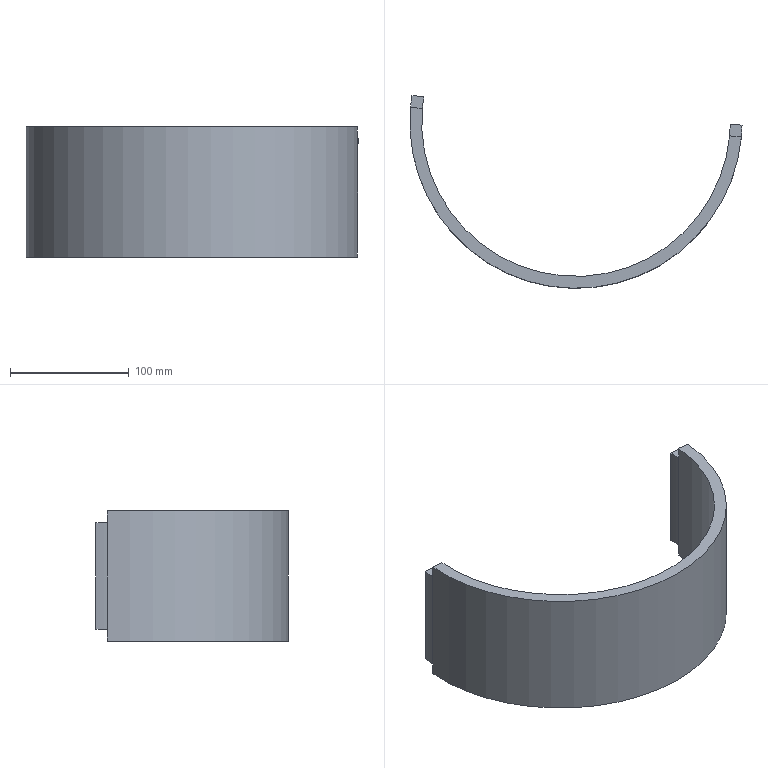Part | SolidWorks | features BaseBody 1 | 1 solid | 18 faces | box 279.978 x 162.405 x 110 mm | volume 484543 mm3 | plane 12 | cylinder 6 | commonest cylinder face diameters 260 x3 280 x3
STEP:
#1=CARTESIAN_POINT('',(399.859,1040.663,-284.893));
#2=VERTEX_POINT('',#1);
#3=CARTESIAN_POINT('',(389.899,1041.555,-284.893));
#4=VERTEX_POINT('',#3);
#5=CARTESIAN_POINT('',(946.393,991.761,-284.893));
#6=DIRECTION('',(-0.996,0.08912,0.));
#7=VECTOR('',#6,1000.);
#8=LINE('',#5,#7);
#9=EDGE_CURVE('',#2,#4,#8,.T.);
#10=ORIENTED_EDGE('',*,*,#9,.F.);
#11=CARTESIAN_POINT('',(399.859,1040.663,-294.893));
#12=VERTEX_POINT('',#11);
#13=CARTESIAN_POINT('',(399.859,1040.663,-184.893));
#14=DIRECTION('',(0.,0.,-1.));
#15=VECTOR('',#14,1000.);
#16=LINE('',#13,#15);
#17=EDGE_CURVE('',#2,#12,#16,.T.);
#18=ORIENTED_EDGE('',*,*,#17,.T.);
#19=CARTESIAN_POINT('',(389.899,1041.555,-294.893));
#20=VERTEX_POINT('',#19);
#21=CARTESIAN_POINT('',(260.416,1053.14,-294.893));
#22=DIRECTION('',(-0.996,0.08912,0.));
#23=VECTOR('',#22,1000.);
#24=LINE('',#21,#23);
#25=EDGE_CURVE('',#12,#20,#24,.T.);
#26=ORIENTED_EDGE('',*,*,#25,.T.);
#27=CARTESIAN_POINT('',(389.899,1041.555,-184.893));
#28=DIRECTION('',(0.,0.,-1.));
#29=VECTOR('',#28,1000.);
#30=LINE('',#27,#29);
#31=EDGE_CURVE('',#4,#20,#30,.T.);
#32=ORIENTED_EDGE('',*,*,#31,.F.);
#33=EDGE_LOOP('',(#10,#18,#26,#32));
#34=FACE_OUTER_BOUND('',#33,.T.);
#35=CARTESIAN_POINT('',(946.393,991.761,-284.893));
#36=DIRECTION('',(0.08912,0.996,0.));
#37=DIRECTION('',(0.,0.,-1.));
#38=AXIS2_PLACEMENT_3D('',#35,#36,#37);
#39=PLANE('',#38);
#40=ADVANCED_FACE('',(#34),#39,.T.);
#41=CARTESIAN_POINT('',(400.394,1050.655,-284.893));
#42=VERTEX_POINT('',#41);
#43=CARTESIAN_POINT('',(390.406,1051.549,-284.893));
#44=VERTEX_POINT('',#43);
#45=CARTESIAN_POINT('',(947.285,1001.721,-284.893));
#46=DIRECTION('',(-0.996,0.08912,0.));
#47=VECTOR('',#46,1000.);
#48=LINE('',#45,#47);
#49=EDGE_CURVE('',#42,#44,#48,.T.);
#50=ORIENTED_EDGE('',*,*,#49,.F.);
#51=CARTESIAN_POINT('',(260.416,1053.14,-284.893));
#52=DIRECTION('',(0.,0.,-1.));
#53=DIRECTION('',(0.08912,0.996,0.));
#54=AXIS2_PLACEMENT_3D('',#51,#52,#53);
#55=CIRCLE('',#54,140.);
#56=EDGE_CURVE('',#42,#2,#55,.T.);
#57=ORIENTED_EDGE('',*,*,#56,.T.);
#58=ORIENTED_EDGE('',*,*,#9,.T.);
#59=CARTESIAN_POINT('',(260.416,1053.14,-284.893));
#60=DIRECTION('',(0.,0.,-1.));
#61=DIRECTION('',(0.08912,0.996,0.));
#62=AXIS2_PLACEMENT_3D('',#59,#60,#61);
#63=CIRCLE('',#62,130.);
#64=EDGE_CURVE('',#44,#4,#63,.T.);
#65=ORIENTED_EDGE('',*,*,#64,.F.);
#66=EDGE_LOOP('',(#50,#57,#58,#65));
#67=FACE_OUTER_BOUND('',#66,.T.);
#68=CARTESIAN_POINT('',(946.393,991.761,-284.893));
#69=DIRECTION('',(0.,0.,-1.));
#70=DIRECTION('',(0.,-1.,0.));
#71=AXIS2_PLACEMENT_3D('',#68,#69,#70);
#72=PLANE('',#71);
#73=ADVANCED_FACE('',(#67),#72,.T.);
#74=CARTESIAN_POINT('',(400.394,1050.655,-194.893));
#75=VERTEX_POINT('',#74);
#76=CARTESIAN_POINT('',(390.406,1051.549,-194.893));
#77=VERTEX_POINT('',#76);
#78=CARTESIAN_POINT('',(947.285,1001.721,-194.893));
#79=DIRECTION('',(-0.996,0.08912,0.));
#80=VECTOR('',#79,1000.);
#81=LINE('',#78,#80);
#82=EDGE_CURVE('',#75,#77,#81,.T.);
#83=ORIENTED_EDGE('',*,*,#82,.F.);
#84=CARTESIAN_POINT('',(400.394,1050.655,-184.893));
#85=DIRECTION('',(0.,0.,-1.));
#86=VECTOR('',#85,1000.);
#87=LINE('',#84,#86);
#88=EDGE_CURVE('',#75,#42,#87,.T.);
#89=ORIENTED_EDGE('',*,*,#88,.T.);
#90=ORIENTED_EDGE('',*,*,#49,.T.);
#91=CARTESIAN_POINT('',(390.406,1051.549,-184.893));
#92=DIRECTION('',(0.,0.,-1.));
#93=VECTOR('',#92,1000.);
#94=LINE('',#91,#93);
#95=EDGE_CURVE('',#77,#44,#94,.T.);
#96=ORIENTED_EDGE('',*,*,#95,.F.);
#97=EDGE_LOOP('',(#83,#89,#90,#96));
#98=FACE_OUTER_BOUND('',#97,.T.);
#99=CARTESIAN_POINT('',(947.285,1001.721,-194.893));
#100=DIRECTION('',(0.08912,0.996,0.));
#101=DIRECTION('',(0.,0.,-1.));
#102=AXIS2_PLACEMENT_3D('',#99,#100,#101);
#103=PLANE('',#102);
#104=ADVANCED_FACE('',(#98),#103,.T.);
#105=CARTESIAN_POINT('',(399.859,1040.663,-194.893));
#106=VERTEX_POINT('',#105);
#107=CARTESIAN_POINT('',(389.899,1041.555,-194.893));
#108=VERTEX_POINT('',#107);
#109=CARTESIAN_POINT('',(946.393,991.761,-194.893));
#110=DIRECTION('',(-0.996,0.08912,0.));
#111=VECTOR('',#110,1000.);
#112=LINE('',#109,#111);
#113=EDGE_CURVE('',#106,#108,#112,.T.);
#114=ORIENTED_EDGE('',*,*,#113,.F.);
#115=CARTESIAN_POINT('',(260.416,1053.14,-194.893));
#116=DIRECTION('',(0.,0.,1.));
#117=DIRECTION('',(0.996,-0.08912,0.));
#118=AXIS2_PLACEMENT_3D('',#115,#116,#117);
#119=CIRCLE('',#118,140.);
#120=EDGE_CURVE('',#106,#75,#119,.T.);
#121=ORIENTED_EDGE('',*,*,#120,.T.);
#122=ORIENTED_EDGE('',*,*,#82,.T.);
#123=CARTESIAN_POINT('',(260.416,1053.14,-194.893));
#124=DIRECTION('',(0.,0.,1.));
#125=DIRECTION('',(0.996,-0.08912,0.));
#126=AXIS2_PLACEMENT_3D('',#123,#124,#125);
#127=CIRCLE('',#126,130.);
#128=EDGE_CURVE('',#108,#77,#127,.T.);
#129=ORIENTED_EDGE('',*,*,#128,.F.);
#130=EDGE_LOOP('',(#114,#121,#122,#129));
#131=FACE_OUTER_BOUND('',#130,.T.);
#132=CARTESIAN_POINT('',(947.285,1001.721,-194.893));
#133=DIRECTION('',(0.,0.,1.));
#134=DIRECTION('',(1.,0.,0.));
#135=AXIS2_PLACEMENT_3D('',#132,#133,#134);
#136=PLANE('',#135);
#137=ADVANCED_FACE('',(#131),#136,.T.);
#138=CARTESIAN_POINT('',(399.859,1040.663,-184.893));
#139=VERTEX_POINT('',#138);
#140=CARTESIAN_POINT('',(389.899,1041.555,-184.893));
#141=VERTEX_POINT('',#140);
#142=CARTESIAN_POINT('',(260.416,1053.14,-184.893));
#143=DIRECTION('',(-0.996,0.08912,0.));
#144=VECTOR('',#143,1000.);
#145=LINE('',#142,#144);
#146=EDGE_CURVE('',#139,#141,#145,.T.);
#147=ORIENTED_EDGE('',*,*,#146,.F.);
#148=CARTESIAN_POINT('',(399.859,1040.663,-184.893));
#149=DIRECTION('',(0.,0.,-1.));
#150=VECTOR('',#149,1000.);
#151=LINE('',#148,#150);
#152=EDGE_CURVE('',#139,#106,#151,.T.);
#153=ORIENTED_EDGE('',*,*,#152,.T.);
#154=ORIENTED_EDGE('',*,*,#113,.T.);
#155=CARTESIAN_POINT('',(389.899,1041.555,-184.893));
#156=DIRECTION('',(0.,0.,-1.));
#157=VECTOR('',#156,1000.);
#158=LINE('',#155,#157);
#159=EDGE_CURVE('',#141,#108,#158,.T.);
#160=ORIENTED_EDGE('',*,*,#159,.F.);
#161=EDGE_LOOP('',(#147,#153,#154,#160));
#162=FACE_OUTER_BOUND('',#161,.T.);
#163=CARTESIAN_POINT('',(946.393,991.761,-112.946));
#164=DIRECTION('',(0.08912,0.996,0.));
#165=DIRECTION('',(0.,0.,-1.));
#166=AXIS2_PLACEMENT_3D('',#163,#164,#165);
#167=PLANE('',#166);
#168=ADVANCED_FACE('',(#162),#167,.T.);
#169=CARTESIAN_POINT('',(130.933,1064.726,-194.893));
#170=VERTEX_POINT('',#169);
#171=CARTESIAN_POINT('',(120.973,1065.617,-194.893));
#172=VERTEX_POINT('',#171);
#173=CARTESIAN_POINT('',(946.393,991.761,-194.893));
#174=DIRECTION('',(-0.996,0.08912,0.));
#175=VECTOR('',#174,1000.);
#176=LINE('',#173,#175);
#177=EDGE_CURVE('',#170,#172,#176,.T.);
#178=ORIENTED_EDGE('',*,*,#177,.T.);
#179=CARTESIAN_POINT('',(120.973,1065.617,-184.893));
#180=VERTEX_POINT('',#179);
#181=CARTESIAN_POINT('',(120.973,1065.617,-184.893));
#182=DIRECTION('',(0.,0.,1.));
#183=VECTOR('',#182,1000.);
#184=LINE('',#181,#183);
#185=EDGE_CURVE('',#172,#180,#184,.T.);
#186=ORIENTED_EDGE('',*,*,#185,.T.);
#187=CARTESIAN_POINT('',(130.933,1064.726,-184.893));
#188=VERTEX_POINT('',#187);
#189=CARTESIAN_POINT('',(260.416,1053.14,-184.893));
#190=DIRECTION('',(-0.996,0.08912,0.));
#191=VECTOR('',#190,1000.);
#192=LINE('',#189,#191);
#193=EDGE_CURVE('',#188,#180,#192,.T.);
#194=ORIENTED_EDGE('',*,*,#193,.F.);
#195=CARTESIAN_POINT('',(130.933,1064.726,-184.893));
#196=DIRECTION('',(0.,0.,1.));
#197=VECTOR('',#196,1000.);
#198=LINE('',#195,#197);
#199=EDGE_CURVE('',#170,#188,#198,.T.);
#200=ORIENTED_EDGE('',*,*,#199,.F.);
#201=EDGE_LOOP('',(#178,#186,#194,#200));
#202=FACE_OUTER_BOUND('',#201,.T.);
#203=CARTESIAN_POINT('',(946.393,991.761,-112.946));
#204=DIRECTION('',(0.08912,0.996,0.));
#205=DIRECTION('',(0.,0.,-1.));
#206=AXIS2_PLACEMENT_3D('',#203,#204,#205);
#207=PLANE('',#206);
#208=ADVANCED_FACE('',(#202),#207,.T.);
#209=CARTESIAN_POINT('',(132.208,1074.652,-194.893));
#210=VERTEX_POINT('',#209);
#211=CARTESIAN_POINT('',(122.22,1075.546,-194.893));
#212=VERTEX_POINT('',#211);
#213=CARTESIAN_POINT('',(947.285,1001.721,-194.893));
#214=DIRECTION('',(-0.996,0.08912,0.));
#215=VECTOR('',#214,1000.);
#216=LINE('',#213,#215);
#217=EDGE_CURVE('',#210,#212,#216,.T.);
#218=ORIENTED_EDGE('',*,*,#217,.T.);
#219=CARTESIAN_POINT('',(260.416,1053.14,-194.893));
#220=DIRECTION('',(0.,0.,1.));
#221=DIRECTION('',(0.996,-0.08912,0.));
#222=AXIS2_PLACEMENT_3D('',#219,#220,#221);
#223=CIRCLE('',#222,140.);
#224=EDGE_CURVE('',#212,#172,#223,.T.);
#225=ORIENTED_EDGE('',*,*,#224,.T.);
#226=ORIENTED_EDGE('',*,*,#177,.F.);
#227=CARTESIAN_POINT('',(260.416,1053.14,-194.893));
#228=DIRECTION('',(0.,0.,1.));
#229=DIRECTION('',(0.996,-0.08912,0.));
#230=AXIS2_PLACEMENT_3D('',#227,#228,#229);
#231=CIRCLE('',#230,130.);
#232=EDGE_CURVE('',#210,#170,#231,.T.);
#233=ORIENTED_EDGE('',*,*,#232,.F.);
#234=EDGE_LOOP('',(#218,#225,#226,#233));
#235=FACE_OUTER_BOUND('',#234,.T.);
#236=CARTESIAN_POINT('',(947.285,1001.721,-194.893));
#237=DIRECTION('',(0.,0.,1.));
#238=DIRECTION('',(1.,0.,0.));
#239=AXIS2_PLACEMENT_3D('',#236,#237,#238);
#240=PLANE('',#239);
#241=ADVANCED_FACE('',(#235),#240,.T.);
#242=CARTESIAN_POINT('',(132.208,1074.652,-284.893));
#243=VERTEX_POINT('',#242);
#244=CARTESIAN_POINT('',(122.22,1075.546,-284.893));
#245=VERTEX_POINT('',#244);
#246=CARTESIAN_POINT('',(947.285,1001.721,-284.893));
#247=DIRECTION('',(-0.996,0.08912,0.));
#248=VECTOR('',#247,1000.);
#249=LINE('',#246,#248);
#250=EDGE_CURVE('',#243,#245,#249,.T.);
#251=ORIENTED_EDGE('',*,*,#250,.T.);
#252=CARTESIAN_POINT('',(122.22,1075.546,-184.893));
#253=DIRECTION('',(0.,0.,1.));
#254=VECTOR('',#253,1000.);
#255=LINE('',#252,#254);
#256=EDGE_CURVE('',#245,#212,#255,.T.);
#257=ORIENTED_EDGE('',*,*,#256,.T.);
#258=ORIENTED_EDGE('',*,*,#217,.F.);
#259=CARTESIAN_POINT('',(132.208,1074.652,-184.893));
#260=DIRECTION('',(0.,0.,1.));
#261=VECTOR('',#260,1000.);
#262=LINE('',#259,#261);
#263=EDGE_CURVE('',#243,#210,#262,.T.);
#264=ORIENTED_EDGE('',*,*,#263,.F.);
#265=EDGE_LOOP('',(#251,#257,#258,#264));
#266=FACE_OUTER_BOUND('',#265,.T.);
#267=CARTESIAN_POINT('',(947.285,1001.721,-194.893));
#268=DIRECTION('',(0.08912,0.996,0.));
#269=DIRECTION('',(0.,0.,-1.));
#270=AXIS2_PLACEMENT_3D('',#267,#268,#269);
#271=PLANE('',#270);
#272=ADVANCED_FACE('',(#266),#271,.T.);
#273=CARTESIAN_POINT('',(130.933,1064.726,-284.893));
#274=VERTEX_POINT('',#273);
#275=CARTESIAN_POINT('',(120.973,1065.617,-284.893));
#276=VERTEX_POINT('',#275);
#277=CARTESIAN_POINT('',(946.393,991.761,-284.893));
#278=DIRECTION('',(-0.996,0.08912,0.));
#279=VECTOR('',#278,1000.);
#280=LINE('',#277,#279);
#281=EDGE_CURVE('',#274,#276,#280,.T.);
#282=ORIENTED_EDGE('',*,*,#281,.T.);
#283=CARTESIAN_POINT('',(260.416,1053.14,-284.893));
#284=DIRECTION('',(0.,0.,-1.));
#285=DIRECTION('',(0.08912,0.996,0.));
#286=AXIS2_PLACEMENT_3D('',#283,#284,#285);
#287=CIRCLE('',#286,140.);
#288=EDGE_CURVE('',#276,#245,#287,.T.);
#289=ORIENTED_EDGE('',*,*,#288,.T.);
#290=ORIENTED_EDGE('',*,*,#250,.F.);
#291=CARTESIAN_POINT('',(260.416,1053.14,-284.893));
#292=DIRECTION('',(0.,0.,-1.));
#293=DIRECTION('',(0.08912,0.996,0.));
#294=AXIS2_PLACEMENT_3D('',#291,#292,#293);
#295=CIRCLE('',#294,130.);
#296=EDGE_CURVE('',#274,#243,#295,.T.);
#297=ORIENTED_EDGE('',*,*,#296,.F.);
#298=EDGE_LOOP('',(#282,#289,#290,#297));
#299=FACE_OUTER_BOUND('',#298,.T.);
#300=CARTESIAN_POINT('',(946.393,991.761,-284.893));
#301=DIRECTION('',(0.,0.,-1.));
#302=DIRECTION('',(0.,-1.,0.));
#303=AXIS2_PLACEMENT_3D('',#300,#301,#302);
#304=PLANE('',#303);
#305=ADVANCED_FACE('',(#299),#304,.T.);
#306=CARTESIAN_POINT('',(130.933,1064.726,-294.893));
#307=VERTEX_POINT('',#306);
#308=CARTESIAN_POINT('',(120.973,1065.617,-294.893));
#309=VERTEX_POINT('',#308);
#310=CARTESIAN_POINT('',(260.416,1053.14,-294.893));
#311=DIRECTION('',(-0.996,0.08912,0.));
#312=VECTOR('',#311,1000.);
#313=LINE('',#310,#312);
#314=EDGE_CURVE('',#307,#309,#313,.T.);
#315=ORIENTED_EDGE('',*,*,#314,.T.);
#316=CARTESIAN_POINT('',(120.973,1065.617,-184.893));
#317=DIRECTION('',(0.,0.,1.));
#318=VECTOR('',#317,1000.);
#319=LINE('',#316,#318);
#320=EDGE_CURVE('',#309,#276,#319,.T.);
#321=ORIENTED_EDGE('',*,*,#320,.T.);
#322=ORIENTED_EDGE('',*,*,#281,.F.);
#323=CARTESIAN_POINT('',(130.933,1064.726,-184.893));
#324=DIRECTION('',(0.,0.,1.));
#325=VECTOR('',#324,1000.);
#326=LINE('',#323,#325);
#327=EDGE_CURVE('',#307,#274,#326,.T.);
#328=ORIENTED_EDGE('',*,*,#327,.F.);
#329=EDGE_LOOP('',(#315,#321,#322,#328));
#330=FACE_OUTER_BOUND('',#329,.T.);
#331=CARTESIAN_POINT('',(946.393,991.761,-284.893));
#332=DIRECTION('',(0.08912,0.996,0.));
#333=DIRECTION('',(0.,0.,-1.));
#334=AXIS2_PLACEMENT_3D('',#331,#332,#333);
#335=PLANE('',#334);
#336=ADVANCED_FACE('',(#330),#335,.T.);
#337=CARTESIAN_POINT('',(389.899,1041.555,-184.893));
#338=DIRECTION('',(0.,0.,-1.));
#339=VECTOR('',#338,1000.);
#340=LINE('',#337,#339);
#341=EDGE_CURVE('',#108,#4,#340,.T.);
#342=ORIENTED_EDGE('',*,*,#341,.F.);
#343=ORIENTED_EDGE('',*,*,#128,.T.);
#344=ORIENTED_EDGE('',*,*,#95,.T.);
#345=ORIENTED_EDGE('',*,*,#64,.T.);
#346=EDGE_LOOP('',(#342,#343,#344,#345));
#347=FACE_OUTER_BOUND('',#346,.T.);
#348=CARTESIAN_POINT('',(260.416,1053.14,-184.893));
#349=DIRECTION('',(0.,0.,-1.));
#350=DIRECTION('',(0.996,-0.08912,0.));
#351=AXIS2_PLACEMENT_3D('',#348,#349,#350);
#352=CYLINDRICAL_SURFACE('',#351,130.);
#353=ADVANCED_FACE('',(#347),#352,.F.);
#354=CARTESIAN_POINT('',(120.973,1065.617,-184.893));
#355=DIRECTION('',(0.,0.,-1.));
#356=VECTOR('',#355,1000.);
#357=LINE('',#354,#356);
#358=EDGE_CURVE('',#172,#276,#357,.T.);
#359=ORIENTED_EDGE('',*,*,#358,.F.);
#360=ORIENTED_EDGE('',*,*,#224,.F.);
#361=ORIENTED_EDGE('',*,*,#256,.F.);
#362=ORIENTED_EDGE('',*,*,#288,.F.);
#363=EDGE_LOOP('',(#359,#360,#361,#362));
#364=FACE_OUTER_BOUND('',#363,.T.);
#365=CARTESIAN_POINT('',(260.416,1053.14,-184.893));
#366=DIRECTION('',(0.,0.,-1.));
#367=DIRECTION('',(0.996,-0.08912,0.));
#368=AXIS2_PLACEMENT_3D('',#365,#366,#367);
#369=CYLINDRICAL_SURFACE('',#368,140.);
#370=ADVANCED_FACE('',(#364),#369,.T.);
#371=ORIENTED_EDGE('',*,*,#25,.F.);
#372=CARTESIAN_POINT('',(260.416,1053.14,-294.893));
#373=DIRECTION('',(0.,0.,1.));
#374=DIRECTION('',(0.996,-0.08912,0.));
#375=AXIS2_PLACEMENT_3D('',#372,#373,#374);
#376=CIRCLE('',#375,140.);
#377=EDGE_CURVE('',#309,#12,#376,.T.);
#378=ORIENTED_EDGE('',*,*,#377,.F.);
#379=ORIENTED_EDGE('',*,*,#314,.F.);
#380=CARTESIAN_POINT('',(260.416,1053.14,-294.893));
#381=DIRECTION('',(0.,0.,1.));
#382=DIRECTION('',(0.996,-0.08912,0.));
#383=AXIS2_PLACEMENT_3D('',#380,#381,#382);
#384=CIRCLE('',#383,130.);
#385=EDGE_CURVE('',#307,#20,#384,.T.);
#386=ORIENTED_EDGE('',*,*,#385,.T.);
#387=EDGE_LOOP('',(#371,#378,#379,#386));
#388=FACE_OUTER_BOUND('',#387,.T.);
#389=CARTESIAN_POINT('',(260.416,1053.14,-294.893));
#390=DIRECTION('',(0.,0.,1.));
#391=DIRECTION('',(1.,0.,0.));
#392=AXIS2_PLACEMENT_3D('',#389,#390,#391);
#393=PLANE('',#392);
#394=ADVANCED_FACE('',(#388),#393,.F.);
#395=CARTESIAN_POINT('',(260.416,1053.14,-184.893));
#396=DIRECTION('',(0.,0.,1.));
#397=DIRECTION('',(0.996,-0.08912,0.));
#398=AXIS2_PLACEMENT_3D('',#395,#396,#397);
#399=CIRCLE('',#398,140.);
#400=EDGE_CURVE('',#180,#139,#399,.T.);
#401=ORIENTED_EDGE('',*,*,#400,.T.);
#402=ORIENTED_EDGE('',*,*,#146,.T.);
#403=CARTESIAN_POINT('',(260.416,1053.14,-184.893));
#404=DIRECTION('',(0.,0.,1.));
#405=DIRECTION('',(0.996,-0.08912,0.));
#406=AXIS2_PLACEMENT_3D('',#403,#404,#405);
#407=CIRCLE('',#406,130.);
#408=EDGE_CURVE('',#188,#141,#407,.T.);
#409=ORIENTED_EDGE('',*,*,#408,.F.);
#410=ORIENTED_EDGE('',*,*,#193,.T.);
#411=EDGE_LOOP('',(#401,#402,#409,#410));
#412=FACE_OUTER_BOUND('',#411,.T.);
#413=CARTESIAN_POINT('',(260.416,1053.14,-184.893));
#414=DIRECTION('',(0.,0.,1.));
#415=DIRECTION('',(1.,0.,0.));
#416=AXIS2_PLACEMENT_3D('',#413,#414,#415);
#417=PLANE('',#416);
#418=ADVANCED_FACE('',(#412),#417,.T.);
#419=CARTESIAN_POINT('',(399.859,1040.663,-184.893));
#420=DIRECTION('',(0.,0.,-1.));
#421=VECTOR('',#420,1000.);
#422=LINE('',#419,#421);
#423=EDGE_CURVE('',#106,#2,#422,.T.);
#424=ORIENTED_EDGE('',*,*,#423,.F.);
#425=ORIENTED_EDGE('',*,*,#152,.F.);
#426=ORIENTED_EDGE('',*,*,#400,.F.);
#427=ORIENTED_EDGE('',*,*,#185,.F.);
#428=ORIENTED_EDGE('',*,*,#358,.T.);
#429=ORIENTED_EDGE('',*,*,#320,.F.);
#430=ORIENTED_EDGE('',*,*,#377,.T.);
#431=ORIENTED_EDGE('',*,*,#17,.F.);
#432=EDGE_LOOP('',(#424,#425,#426,#427,#428,#429,#430,#431));
#433=FACE_OUTER_BOUND('',#432,.T.);
#434=CARTESIAN_POINT('',(260.416,1053.14,-184.893));
#435=DIRECTION('',(0.,0.,-1.));
#436=DIRECTION('',(0.996,-0.08912,0.));
#437=AXIS2_PLACEMENT_3D('',#434,#435,#436);
#438=CYLINDRICAL_SURFACE('',#437,140.);
#439=ADVANCED_FACE('',(#433),#438,.T.);
#440=ORIENTED_EDGE('',*,*,#120,.F.);
#441=ORIENTED_EDGE('',*,*,#423,.T.);
#442=ORIENTED_EDGE('',*,*,#56,.F.);
#443=ORIENTED_EDGE('',*,*,#88,.F.);
#444=EDGE_LOOP('',(#440,#441,#442,#443));
#445=FACE_OUTER_BOUND('',#444,.T.);
#446=CARTESIAN_POINT('',(260.416,1053.14,-184.893));
#447=DIRECTION('',(0.,0.,-1.));
#448=DIRECTION('',(0.996,-0.08912,0.));
#449=AXIS2_PLACEMENT_3D('',#446,#447,#448);
#450=CYLINDRICAL_SURFACE('',#449,140.);
#451=ADVANCED_FACE('',(#445),#450,.T.);
#452=ORIENTED_EDGE('',*,*,#232,.T.);
#453=CARTESIAN_POINT('',(130.933,1064.726,-184.893));
#454=DIRECTION('',(0.,0.,-1.));
#455=VECTOR('',#454,1000.);
#456=LINE('',#453,#455);
#457=EDGE_CURVE('',#170,#274,#456,.T.);
#458=ORIENTED_EDGE('',*,*,#457,.T.);
#459=ORIENTED_EDGE('',*,*,#296,.T.);
#460=ORIENTED_EDGE('',*,*,#263,.T.);
#461=EDGE_LOOP('',(#452,#458,#459,#460));
#462=FACE_OUTER_BOUND('',#461,.T.);
#463=CARTESIAN_POINT('',(260.416,1053.14,-184.893));
#464=DIRECTION('',(0.,0.,-1.));
#465=DIRECTION('',(0.996,-0.08912,0.));
#466=AXIS2_PLACEMENT_3D('',#463,#464,#465);
#467=CYLINDRICAL_SURFACE('',#466,130.);
#468=ADVANCED_FACE('',(#462),#467,.F.);
#469=ORIENTED_EDGE('',*,*,#159,.T.);
#470=ORIENTED_EDGE('',*,*,#341,.T.);
#471=ORIENTED_EDGE('',*,*,#31,.T.);
#472=ORIENTED_EDGE('',*,*,#385,.F.);
#473=ORIENTED_EDGE('',*,*,#327,.T.);
#474=ORIENTED_EDGE('',*,*,#457,.F.);
#475=ORIENTED_EDGE('',*,*,#199,.T.);
#476=ORIENTED_EDGE('',*,*,#408,.T.);
#477=EDGE_LOOP('',(#469,#470,#471,#472,#473,#474,#475,#476));
#478=FACE_OUTER_BOUND('',#477,.T.);
#479=CARTESIAN_POINT('',(260.416,1053.14,-184.893));
#480=DIRECTION('',(0.,0.,-1.));
#481=DIRECTION('',(0.996,-0.08912,0.));
#482=AXIS2_PLACEMENT_3D('',#479,#480,#481);
#483=CYLINDRICAL_SURFACE('',#482,130.);
#484=ADVANCED_FACE('',(#478),#483,.F.);
#485=CLOSED_SHELL('',(#40,#73,#104,#137,#168,#208,#241,#272,#305,#336,#353,#370,#394,#418,#439,#451,#468,#484));
#486=MANIFOLD_SOLID_BREP('',#485);
#487=CARTESIAN_POINT('',(0.,0.,0.));
#488=DIRECTION('',(0.,0.,1.));
#489=DIRECTION('',(1.,0.,0.));
#490=AXIS2_PLACEMENT_3D('',#487,#488,#489);
#491=(LENGTH_UNIT()NAMED_UNIT(*)SI_UNIT(.MILLI.,.METRE.));
#492=UNCERTAINTY_MEASURE_WITH_UNIT(LENGTH_MEASURE(0.00001),#491,'','');
#493=(NAMED_UNIT(*)PLANE_ANGLE_UNIT()SI_UNIT($,.RADIAN.));
#494=(NAMED_UNIT(*)SI_UNIT($,.STERADIAN.)SOLID_ANGLE_UNIT());
#495=(GEOMETRIC_REPRESENTATION_CONTEXT(3)GLOBAL_UNCERTAINTY_ASSIGNED_CONTEXT((#492))GLOBAL_UNIT_ASSIGNED_CONTEXT((#491,#493,#494))REPRESENTATION_CONTEXT('',''));
#496=ADVANCED_BREP_SHAPE_REPRESENTATION('',(#486,#490),#495);